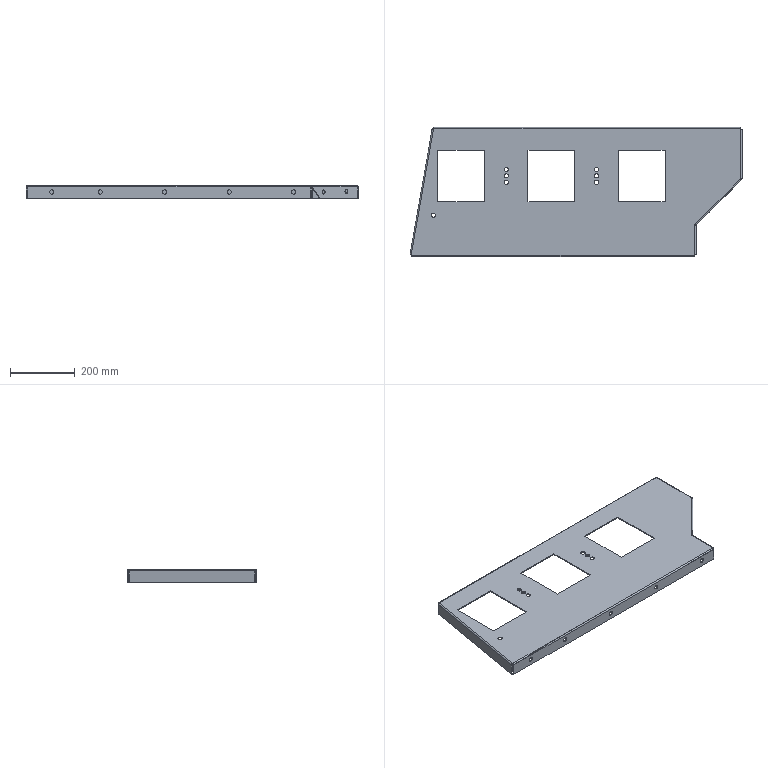Part | SolidWorks | features BaseBody 1 | 1 solid | 108 faces | box 1030 x 400 x 40 mm | volume 1189266 mm3 | plane 62 | cylinder 46 | commonest cylinder face diameters 13 x30 2 x6 8 x6 15 x4